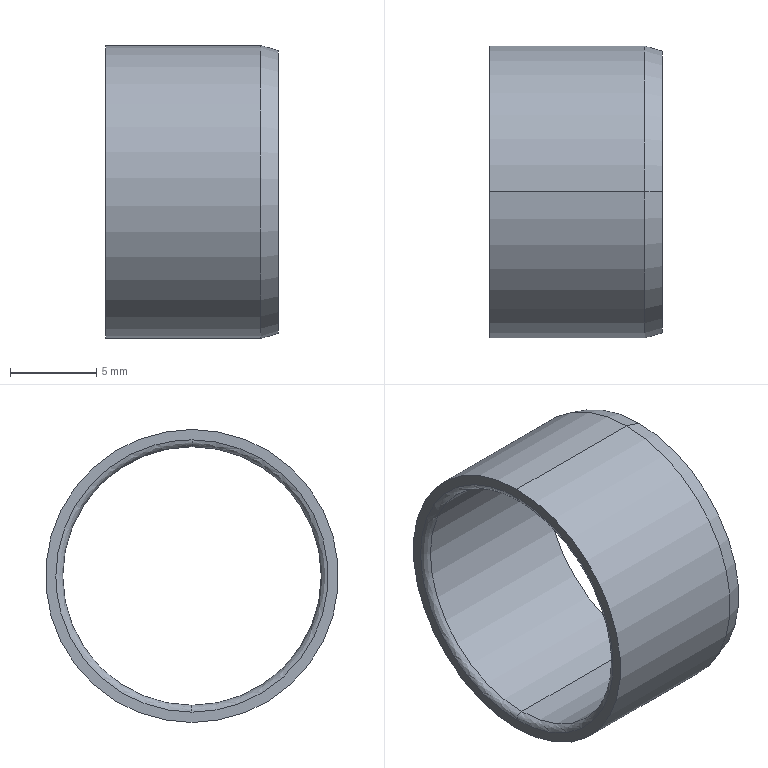Part | STEP file | 0232_008_JZB15-10 | 1 solid | 10 faces | box 10 x 17 x 17 mm | volume 493.192 mm3 | cylinder 4 | spline 2 | cone 2 | plane 2 | commonest cylinder face diameters 15 x2 17 x2